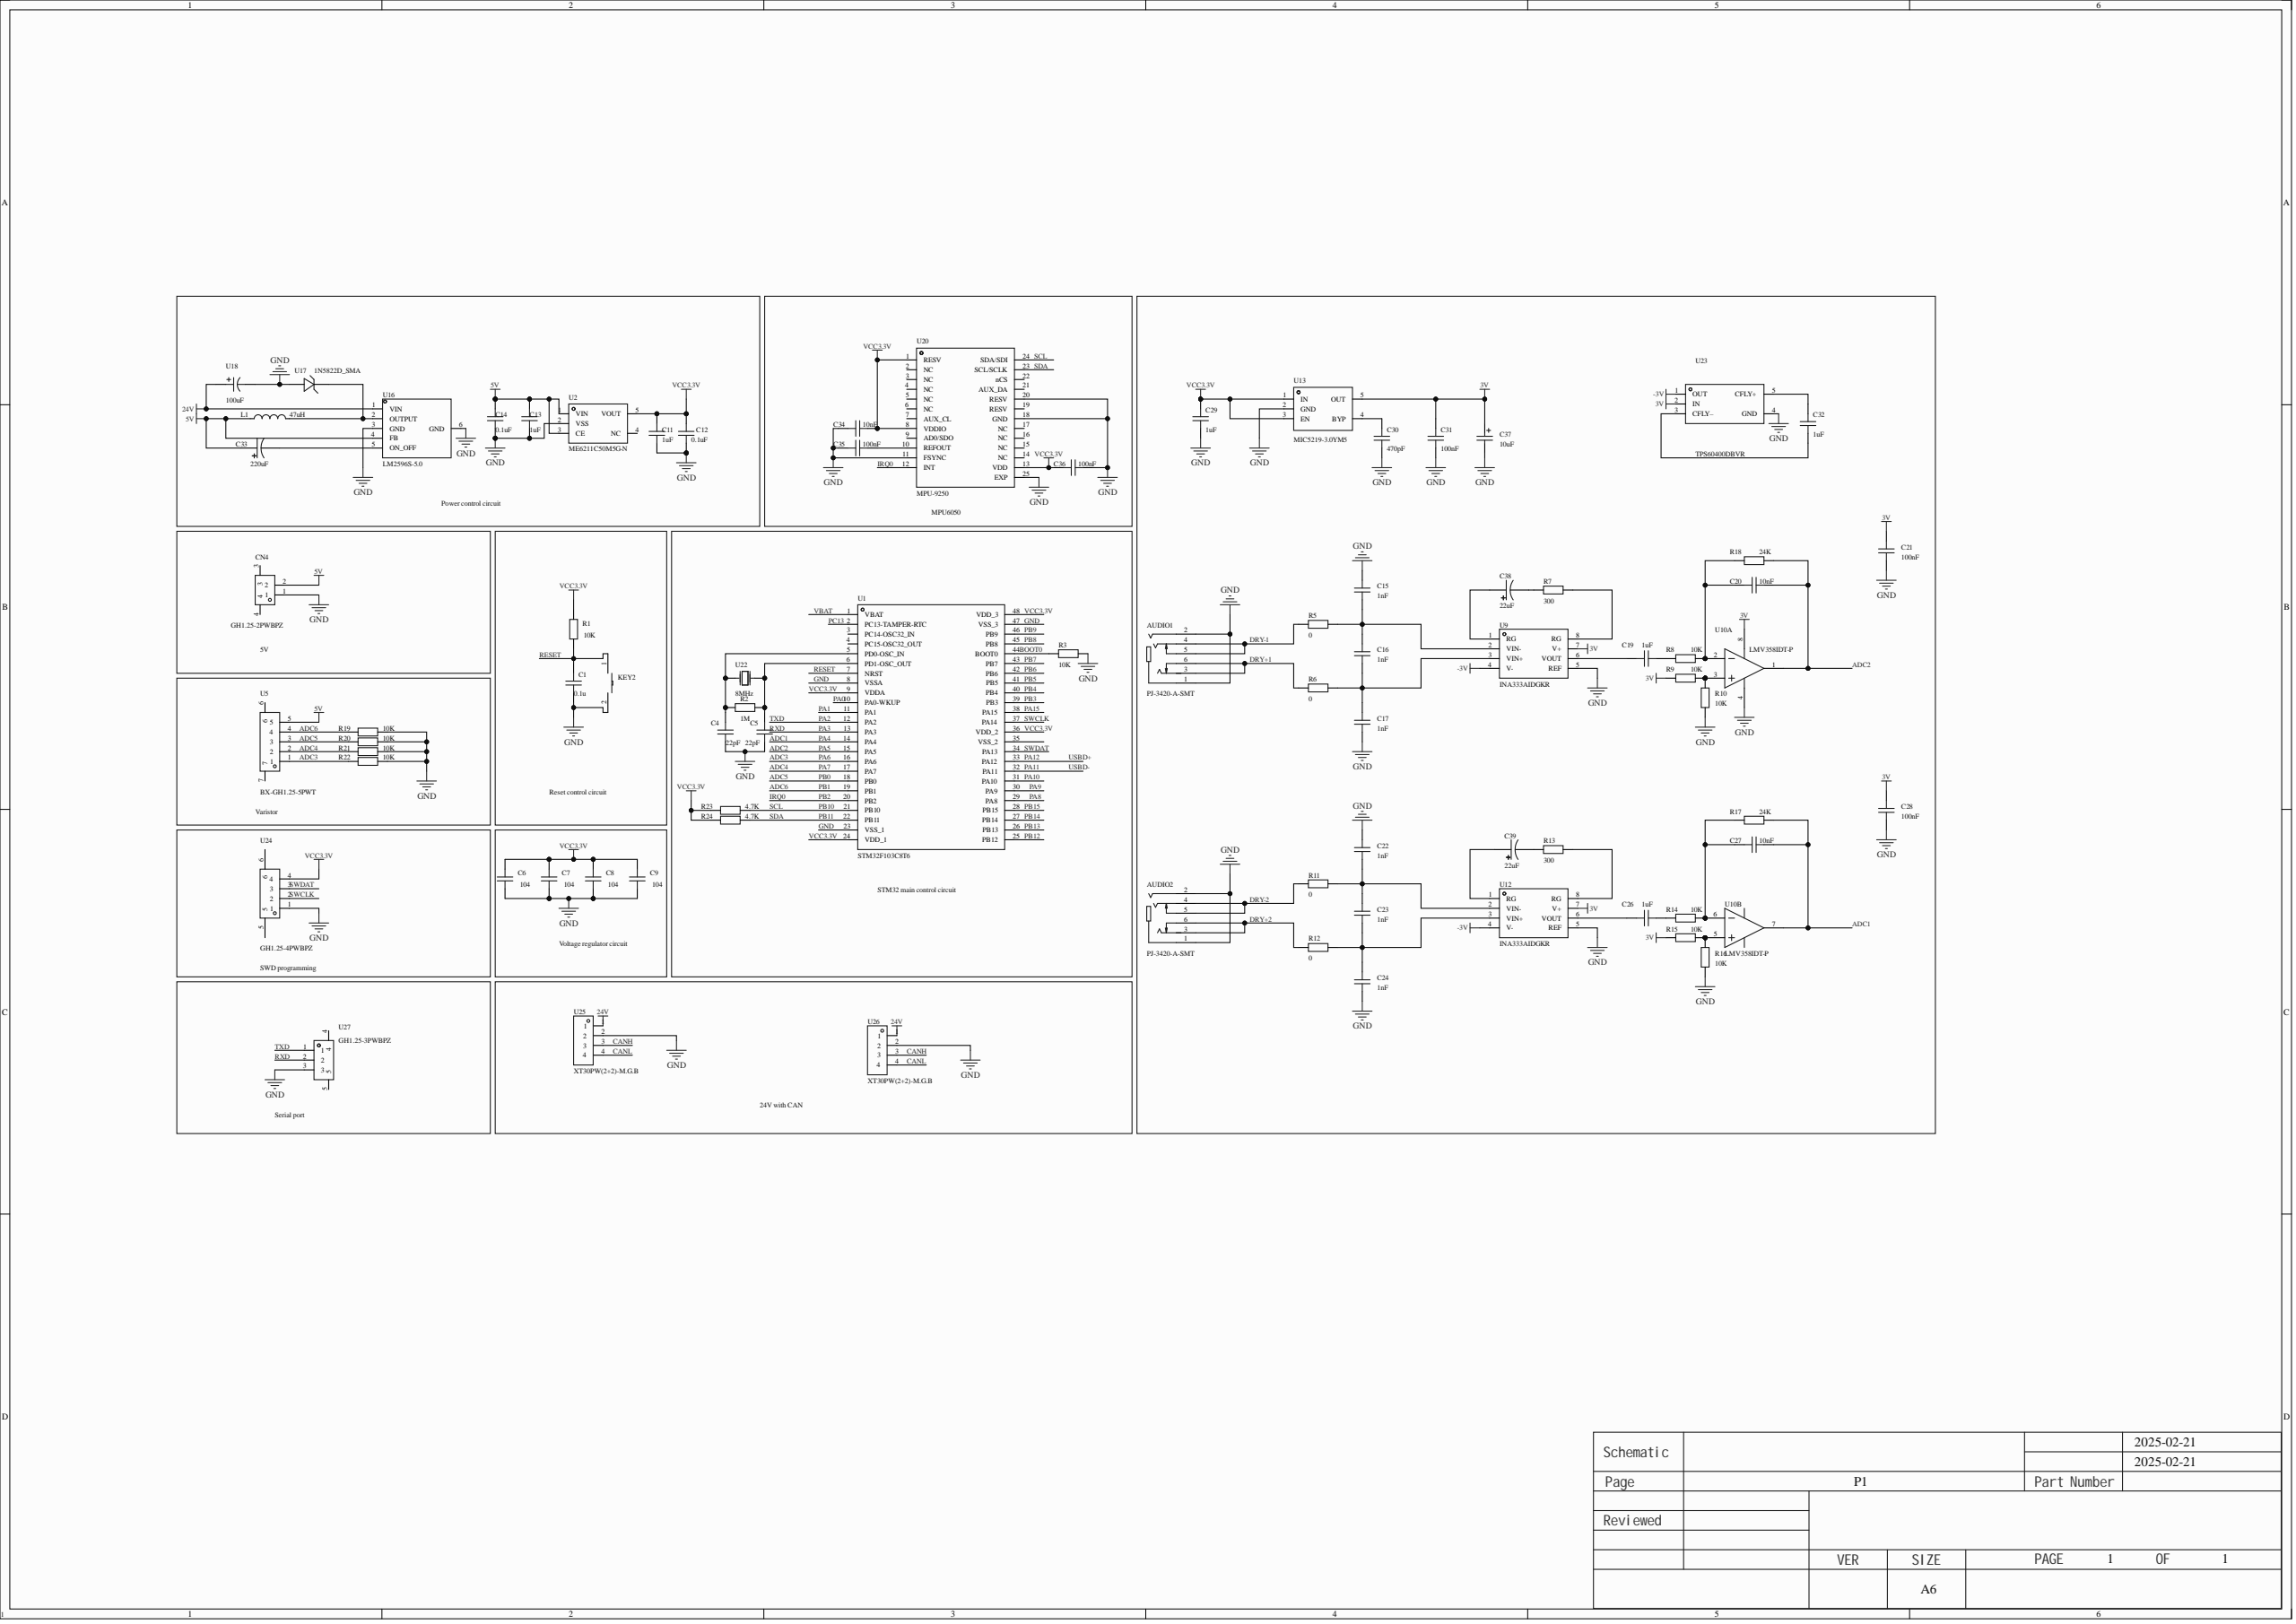Circuit board | Altium Designer | 79 parts | 53 nets
Bill of materials:
Comment,Description,Designator,Footprint,LibRef,Quantity
"PJ-3420-A-SMT","Connector type:3.5mm headphone jack;Rated current:500mA;Rated voltage:30V;Operating temperature range:-20℃~+70℃;Soldering temperature (max):235℃;","AUDIO1, AUDIO2","AUDIO-SMD_PJ-3420-A-SMT_C319102","PJ-3420-A-SMT","2"
"0.1u","","C1","C0603","CAP_0603","1"
"22pF","","C4, C5","C0603","CAP_0603","2"
"104","","C6, C7, C8, C9","C0603","CAP_0603","4"
"1uF","","C11, C13, C19, C26, C29, C32","C0603","CAP_0603","6"
"0.1uF","","C12, C14","C0603","CAP_0603","2"
"1nF","","C15, C16, C17, C22, C23, C24","C0603","CAP_0603","6"
"10nF","","C20, C27, C34","C0603","CAP_0603","3"
"100nF","","C21, C28, C31, C35, C36","C0603","CAP_0603","5"
"470pF","","C30","C0603","CAP_0603","1"
"220uF","Capacitance:220uF;Tolerance:±20%;Rated voltage:35V;Ripple current:755mA@100kHz;Equivalent series resistance:90mO@100kHz;","C33","CAP-TH_BD10.0-P5.00-D1.0-FD","EEUFC1V221B","1"
"10uF","Capacitance:10uF;Tolerance:±10%;Rated voltage:16V;Equivalent series resistance:10O@100kHz;","C37","CAP-SMD_L3.2-W1.6-RD","CA45-A-16V-10uF-K","1"
"22uF","Capacitance:22uF;Tolerance:±20%;Rated voltage:50V;Ripple current:238mA@100kHz;Equivalent series resistance:-;","C38, C39","CAP-SMD_BD5.0-L5.3-W5.3-RD","VKMB1001H220MV","2"
"GH1.25-2PWBPZ","","CN4","CONN-SMD_GH1.25-2PWBPZ","GH1.25-2PWBPZ","1"
"TS-1101-C-W","Contact current:50mA;Rated voltage (DC):12V;Insulation resistance:-;Circuit structure:SPST;Mounting style:Vertical SMT;Button shape:Rectangular button;Button/cap color:White;With lamp:None;Actuation force:260gf;Mechanical life:50000;Operating temperature:-30℃~+85℃;Switch length:6mm;Switch width:3.6mm;Switch height:2.5mm;With bracket:No;","KEY2","SW-SMD_L6.0-W3.3-LS8.0","TS-1101-C-W","1"
"47uH","Inductance:47uH;Tolerance:±20%;Rated current:-;Saturation current (Isat):-;","L1","IND-SMD_L12.3-W12.3","CDRH127N-470M","1"
"10K","","R1, R3, R8, R9, R10, R14, R15, R16, R19, R20, R21, R22","R0603","Res_0603","12"
"1M","","R2","R0603","Res_0603","1"
"0","","R5, R6, R11, R12","R0603","Res_0603","4"
"300","","R7, R13","R0603","Res_0603","2"
"24K","","R17, R18","R0603","Res_0603","2"
"4.7K","","R23, R24","R0603","Res_0603","2"
"STM32F103C8T6","CPU core:ARM Cortex-M3;CPU max frequency:72MHz;Program storage capacity:64KB;Program memory type:FLASH;Total RAM:20KB;GPIO port count:37;ADC (bits):12bit;Operating temperature range:-40℃~+85℃;","U1","LQFP-48_L7.0-W7.0-P0.50-LS9.0-BL","STM32F103C8T6","1"
"ME6211C50M5G-N","-","U2","SOT-23-5_L3.0-W1.7-P0.95-LS2.8-BL","ME6211C50M5G-N","1"
"BX-GH1.25-5PWT","Pin structure:1x5P;Pitch:1.25mm;Mounting style:Horizontal SMT;Reference series:GH;Total pins:5P;Rows:1;Pins per row:5;Row spacing:-;Rated current:1A;Contact material:Phosphor bronze;Contact plating:Tin;Operating temperature:-25℃~+85℃;","U5","CONN-SMD_5P-P1.25_BX-GH1.25-5PWT","BX-GH1.25-5PWT","1"
"INA333AIDGKR","Amplifier count:Single;Input bias current (Ib):70pA;Input offset voltage (Vos):10uV;Slew rate (SR):0.16V/us;Bandwidth (-3dB):150kHz;Rail-to-rail:-;","U9, U12","MSOP-8_L3.0-W3.0-P0.65-LS5.0-BL","INA333AIDGKR","2"
"LMV358IDT-P","Rail-to-rail:Rail-to-rail input, rail-to-rail output;Gain bandwidth product (GBP):1MHz;Input offset voltage (Vos):5mV;Slew rate (SR):0.6V/us;","U10","SOP-8_L4.9-W3.9-P1.27-LS6.0-BL","LMV358IDT-P","1"
"MIC5219-3.0YM5","Output type:Fixed;Max input voltage:12V;Output voltage:3V;Max output current:500mA;Power supply ripple rejection (PSRR):75dB@(120Hz);Output polarity:Positive;","U13","SOT-23-5_L2.9-W1.6-P0.95-LS2.8-BL","MIC5219-3.0YM5-TR","1"
"LM2596S-5.0","Function type:Step-down;Output type:Fixed;Operating voltage:4.5V~30V;Output voltage:5V;Output current:3A;","U16","TO-263-5_L10.1-W8.7-P1.70-LS14.4-BR","LM2596S-5.0","1"
"1N5822D_SMA","","U17","SMA_L4.3-W2.6-LS5.2-RD","1N5822D_SMA","1"
"100uF","","U18","CAP-SMD_L3.5-W2.8-FD","贴片钽电容100uF+-20%6.3VB型","1"
"MPU-9250","9-axis sensor","U20","QFN-24_L3.0-W3.0-P0.40-BL-EP","MPU-9250","1"
"8MHz","Frequency:8MHz;Frequency tolerance at room temperature:±50ppm;External load capacitance:8pF;Frequency stability (full temperature):±150ppm;","U22","OSC-SMD-2P_-L5.0-W3.2","NX5032GA-8.000M-STD-CSU-1","1"
"TPS60400DBVR","TPS60400 60mA charge-pump voltage inverter with variable switching frequency","U23","SOT-23-5_L3.0-W1.7-P0.95-LS2.8-BR","TPS60400DBVR","1"
"GH1.25-4PWBPZ","","U24","CONN-SMD_GH1.25-4PWBPZ","GH1.25-4PWBPZ","1"
"XT30PW(2+2)-M.G.B","","U25, U26","CONN-TH_4P-XT30PW-M","XT30PW(2+2)-M.G.B","2"
"GH1.25-3PWBPZ","","U27","CONN-SMD_GH1.25-3PWBPZ","GH1.25-3PWBPZ","1"
Netlist (Protel format):
[
AUDIO1
AUDIO-SMD_PJ-3420-A-SMT_C319102
PJ-3420-A-SMT



]
[
AUDIO2
AUDIO-SMD_PJ-3420-A-SMT_C319102
PJ-3420-A-SMT



]
[
C1
C0603
0.1u



]
[
C4
C0603
22pF



]
[
C5
C0603
22pF



]
[
C6
C0603
104



]
[
C7
C0603
104



]
[
C8
C0603
104



]
[
C9
C0603
104



]
[
C11
C0603
1uF



]
[
C12
C0603
0.1uF



]
[
C13
C0603
1uF



]
[
C14
C0603
0.1uF



]
[
C15
C0603
1nF



]
[
C16
C0603
1nF



]
[
C17
C0603
1nF



]
[
C19
C0603
1uF



]
[
C20
C0603
10nF



]
[
C21
C0603
100nF



]
[
C22
C0603
1nF



]
[
C23
C0603
1nF



]
[
C24
C0603
1nF



]
[
C26
C0603
1uF



]
[
C27
C0603
10nF



]
[
C28
C0603
100nF



]
[
C29
C0603
1uF



]
[
C30
C0603
470pF



]
[
C31
C0603
100nF



]
[
C32
C0603
1uF



]
[
C33
CAP-TH_BD10.0-P5.00-D1.0-FD
220uF



]
[
C34
C0603
10nF



]
[
C35
C0603
100nF



]
[
C36
C0603
100nF



]
[
C37
CAP-SMD_L3.2-W1.6-RD
10uF



]
[
C38
CAP-SMD_BD5.0-L5.3-W5.3-RD
22uF



]
[
C39
CAP-SMD_BD5.0-L5.3-W5.3-RD
22uF



]
[
CN4
CONN-SMD_GH1.25-2PWBPZ
GH1.25-2PWBPZ



]
[
KEY2
SW-SMD_L6.0-W3.3-LS8.0
TS-1101-C-W



]
[
L1
IND-SMD_L12.3-W12.3
47uH



]
[
R1
R0603
10K



]
[
R2
R0603
1M



]
[
R3
R0603
10K



]
[
R5
R0603
0



]
[
R6
R0603
0



]
[
R7
R0603
300



]
[
R8
R0603
10K



]
[
R9
R0603
10K



]
[
R10
R0603
10K



]
[
R11
R0603
0



]
[
R12
R0603
0



]
[
R13
R0603
300



]
[
R14
R0603
10K



]
[
R15
R0603
10K



]
[
R16
R0603
10K



]
[
R17
R0603
24K



]
[
R18
R0603
24K



]
[
R19
R0603
10K



]
[
R20
R0603
10K



]
[
R21
R0603
10K



]
[
R22
R0603
10K



]
[
R23
R0603
4.7K



]
[
R24
R0603
4.7K



]
[
U1
LQFP-48_L7.0-W7.0-P0.50-LS9.0-BL
STM32F103C8T6



]
[
U2
SOT-23-5_L3.0-W1.7-P0.95-LS2.8-BL
ME6211C50M5G-N



]
[
U5
CONN-SMD_5P-P1.25_BX-GH1.25-5PWT
BX-GH1.25-5PWT



]
[
U9
MSOP-8_L3.0-W3.0-P0.65-LS5.0-BL
INA333AIDGKR



]
[
U10
SOP-8_L4.9-W3.9-P1.27-LS6.0-BL
LMV358IDT-P



]
[
U12
MSOP-8_L3.0-W3.0-P0.65-LS5.0-BL
INA333AIDGKR



]
[
U13
SOT-23-5_L2.9-W1.6-P0.95-LS2.8-BL
MIC5219-3.0YM5



]
[
U16
TO-263-5_L10.1-W8.7-P1.70-LS14.4-BR
LM2596S-5.0



]
[
U17
SMA_L4.3-W2.6-LS5.2-RD
1N5822D_SMA



]
[
U18
CAP-SMD_L3.5-W2.8-FD
100uF



]
[
U20
QFN-24_L3.0-W3.0-P0.40-BL-EP
MPU-9250



]
[
U22
OSC-SMD-2P_-L5.0-W3.2
8MHz



]
[
U23
SOT-23-5_L3.0-W1.7-P0.95-LS2.8-BR
TPS60400DBVR



]
[
U24
CONN-SMD_GH1.25-4PWBPZ
GH1.25-4PWBPZ



]
[
U25
CONN-TH_4P-XT30PW-M
XT30PW(2+2)-M.G.B



]
[
U26
CONN-TH_4P-XT30PW-M
XT30PW(2+2)-M.G.B



]
[
U27
CONN-SMD_GH1.25-3PWBPZ
GH1.25-3PWBPZ



]
(
VCC3.3V
C6-2
C7-2
C8-2
C9-2
C11-2
C12-2
C29-1
C34-1
C36-1
R1-2
R23-1
R24-1
U1-9
U1-24
U1-36
U1-48
U2-5
U13-1
U13-3
U20-1
U20-8
U20-13
U24-4
)
(
SWDAT
U1-34
U24-3
)
(
SWCLK
U1-37
U24-2
)
(
RESET
C1-2
KEY2-1
R1-1
U1-7
)
(
PB11
R24-2
U1-22
U20-23
)
(
PB10
R23-2
U1-21
U20-24
)
(
PA3
U1-13
U27-2
)
(
PA2
U1-12
U27-1
)
(
NetR15_2
R15-2
R16-2
U10-5
)
(
NetR13_2
R13-2
U12-8
)
(
NetR9_2
R9-2
R10-2
U10-3
)
(
NetR7_2
R7-2
U9-8
)
(
NetL1_2
L1-2
U16-2
U17-1
)
(
NetC39_2
C39-2
R13-1
)
(
NetC39_1
C39-1
U12-1
)
(
NetC38_2
C38-2
R7-1
)
(
NetC38_1
C38-1
U9-1
)
(
NetC35_1
C35-1
U20-10
)
(
NetC33_2
C33-2
U16-5
)
(
NetC32_2
C32-2
U23-3
)
(
NetC32_1
C32-1
U23-5
)
(
NetC30_1
C30-1
U13-4
)
(
NetC27_2
C27-2
R14-2
R17-1
U10-6
)
(
NetC26_2
C26-2
U12-6
)
(
NetC26_1
C26-1
R14-1
)
(
NetC23_1
C23-1
C24-2
R12-2
U12-3
)
(
NetC22_1
C22-1
C23-2
R11-2
U12-2
)
(
NetC20_2
C20-2
R8-2
R18-1
U10-2
)
(
NetC19_2
C19-2
U9-6
)
(
NetC19_1
C19-1
R8-1
)
(
NetC16_1
C16-1
C17-2
R6-2
U9-3
)
(
NetC15_1
C15-1
C16-2
R5-2
U9-2
)
(
NetC5_2
C5-2
R2-2
U1-6
U22-2
)
(
NetC4_2
C4-2
R2-1
U1-5
U22-1
)
(
IRQ0
U1-20
U20-12
)
(
GND
AUDIO1-1
AUDIO1-2
AUDIO2-1
AUDIO2-2
C1-1
C4-1
C5-1
C6-1
C7-1
C8-1
C9-1
C11-1
C12-1
C13-1
C14-1
C15-2
C17-1
C21-2
C22-2
C24-1
C28-2
C29-2
C30-2
C31-2
C34-2
C35-2
C36-2
C37-2
CN4-1
KEY2-2
R3-2
R10-1
R16-1
R19-1
R20-1
R21-1
R22-1
U1-8
U1-23
U1-47
U2-2
U9-5
U10-4
U12-5
U13-2
U16-3
U16-6
U17-2
U18-2
U20-11
U20-18
U20-20
U20-25
U23-4
U24-1
U25-2
U26-2
U27-3
)
(
DRY-2
AUDIO2-4
AUDIO2-5
R11-1
)
(
DRY-1
AUDIO1-4
AUDIO1-5
R5-1
)
(
DRY+2
AUDIO2-3
AUDIO2-6
R12-1
)
(
DRY+1
AUDIO1-3
AUDIO1-6
R6-1
)
(
CANL
U25-4
U26-4
)
(
CANH
U25-3
U26-3
)
(
BOOT0
R3-1
U1-44
)
(
ADC6
R19-2
U1-19
U5-4
)
(
ADC5
R20-2
U1-18
U5-3
)
(
ADC4
R21-2
U1-17
U5-2
)
(
ADC3
R22-2
U1-16
U5-1
)
(
ADC2
C20-1
R18-2
U1-15
U10-1
)
(
ADC1
C27-1
R17-2
U1-14
U10-7
)
(
-3V
U9-4
U12-4
U23-1
)
(
24V
U16-1
U18-1
U25-1
U26-1
)
(
5V
C13-2
C14-2
C33-1
CN4-2
L1-1
U2-1
U2-3
U5-5
U16-4
)
(
3V
C21-1
C28-1
C31-1
C37-1
R9-1
R15-1
U9-7
U10-8
U12-7
U13-5
U23-2
)